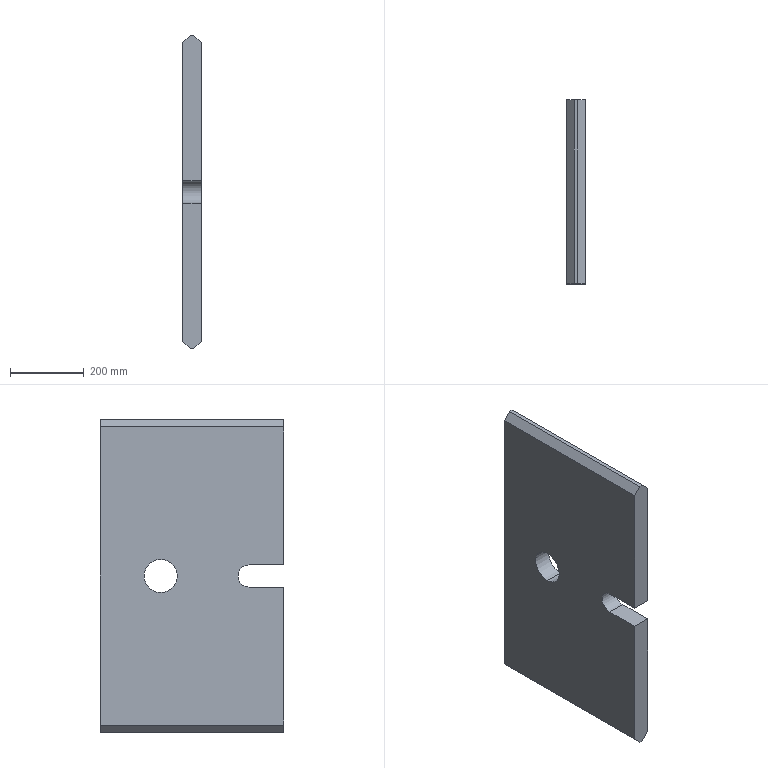Part | SolidWorks | features Chamfer 1, Extrusion 1 | 1 solid | 16 faces | box 50 x 500 x 850 mm | volume 20176228 mm3 | plane 13 | cylinder 3 | commonest cylinder face diameters 90 x2 60 x1
STEP:
#1=CARTESIAN_POINT('',(25.,85.,45.));
#2=VERTEX_POINT('',#1);
#3=CARTESIAN_POINT('',(25.,85.,-45.));
#4=VERTEX_POINT('',#3);
#5=CARTESIAN_POINT('',(25.,85.,0.));
#6=DIRECTION('',(1.,0.,0.));
#7=DIRECTION('',(0.,0.,-1.));
#8=AXIS2_PLACEMENT_3D('',#5,#6,#7);
#9=CIRCLE('',#8,45.);
#10=EDGE_CURVE('',#2,#4,#9,.T.);
#11=ORIENTED_EDGE('',*,*,#10,.T.);
#12=CARTESIAN_POINT('',(-25.,85.,-45.));
#13=VERTEX_POINT('',#12);
#14=CARTESIAN_POINT('',(25.,85.,-45.));
#15=DIRECTION('',(-1.,0.,0.));
#16=VECTOR('',#15,1000.);
#17=LINE('',#14,#16);
#18=EDGE_CURVE('',#4,#13,#17,.T.);
#19=ORIENTED_EDGE('',*,*,#18,.T.);
#20=CARTESIAN_POINT('',(-25.,85.,45.));
#21=VERTEX_POINT('',#20);
#22=CARTESIAN_POINT('',(-25.,85.,0.));
#23=DIRECTION('',(1.,0.,0.));
#24=DIRECTION('',(0.,0.,-1.));
#25=AXIS2_PLACEMENT_3D('',#22,#23,#24);
#26=CIRCLE('',#25,45.);
#27=EDGE_CURVE('',#21,#13,#26,.T.);
#28=ORIENTED_EDGE('',*,*,#27,.F.);
#29=CARTESIAN_POINT('',(25.,85.,45.));
#30=DIRECTION('',(-1.,0.,0.));
#31=VECTOR('',#30,1000.);
#32=LINE('',#29,#31);
#33=EDGE_CURVE('',#2,#21,#32,.T.);
#34=ORIENTED_EDGE('',*,*,#33,.F.);
#35=EDGE_LOOP('',(#11,#19,#28,#34));
#36=FACE_OUTER_BOUND('',#35,.T.);
#37=CARTESIAN_POINT('',(25.,85.,0.));
#38=DIRECTION('',(-1.,0.,0.));
#39=DIRECTION('',(0.,0.,1.));
#40=AXIS2_PLACEMENT_3D('',#37,#38,#39);
#41=CYLINDRICAL_SURFACE('',#40,45.);
#42=ADVANCED_FACE('',(#36),#41,.F.);
#43=CARTESIAN_POINT('',(25.,-250.,-30.));
#44=VERTEX_POINT('',#43);
#45=CARTESIAN_POINT('',(25.,-250.,-405.));
#46=VERTEX_POINT('',#45);
#47=CARTESIAN_POINT('',(25.,-250.,-425.));
#48=DIRECTION('',(0.,0.,-1.));
#49=VECTOR('',#48,1000.);
#50=LINE('',#47,#49);
#51=EDGE_CURVE('',#44,#46,#50,.T.);
#52=ORIENTED_EDGE('',*,*,#51,.T.);
#53=CARTESIAN_POINT('',(25.,250.,-405.));
#54=VERTEX_POINT('',#53);
#55=CARTESIAN_POINT('',(25.,250.,-405.));
#56=DIRECTION('',(0.,1.,0.));
#57=VECTOR('',#56,1000.);
#58=LINE('',#55,#57);
#59=EDGE_CURVE('',#46,#54,#58,.T.);
#60=ORIENTED_EDGE('',*,*,#59,.T.);
#61=CARTESIAN_POINT('',(25.,250.,405.));
#62=VERTEX_POINT('',#61);
#63=CARTESIAN_POINT('',(25.,250.,-425.));
#64=DIRECTION('',(0.,0.,1.));
#65=VECTOR('',#64,1000.);
#66=LINE('',#63,#65);
#67=EDGE_CURVE('',#54,#62,#66,.T.);
#68=ORIENTED_EDGE('',*,*,#67,.T.);
#69=CARTESIAN_POINT('',(25.,-250.,405.));
#70=VERTEX_POINT('',#69);
#71=CARTESIAN_POINT('',(25.,-250.,405.));
#72=DIRECTION('',(0.,-1.,0.));
#73=VECTOR('',#72,1000.);
#74=LINE('',#71,#73);
#75=EDGE_CURVE('',#62,#70,#74,.T.);
#76=ORIENTED_EDGE('',*,*,#75,.T.);
#77=CARTESIAN_POINT('',(25.,-250.,30.));
#78=VERTEX_POINT('',#77);
#79=CARTESIAN_POINT('',(25.,-250.,30.));
#80=DIRECTION('',(0.,0.,-1.));
#81=VECTOR('',#80,1000.);
#82=LINE('',#79,#81);
#83=EDGE_CURVE('',#70,#78,#82,.T.);
#84=ORIENTED_EDGE('',*,*,#83,.T.);
#85=CARTESIAN_POINT('',(25.,-155.,30.));
#86=VERTEX_POINT('',#85);
#87=CARTESIAN_POINT('',(25.,-155.,30.));
#88=DIRECTION('',(0.,1.,0.));
#89=VECTOR('',#88,1000.);
#90=LINE('',#87,#89);
#91=EDGE_CURVE('',#78,#86,#90,.T.);
#92=ORIENTED_EDGE('',*,*,#91,.T.);
#93=CARTESIAN_POINT('',(25.,-155.,-30.));
#94=VERTEX_POINT('',#93);
#95=CARTESIAN_POINT('',(25.,-155.,0.));
#96=DIRECTION('',(-1.,0.,0.));
#97=DIRECTION('',(0.,0.,-1.));
#98=AXIS2_PLACEMENT_3D('',#95,#96,#97);
#99=CIRCLE('',#98,30.);
#100=EDGE_CURVE('',#86,#94,#99,.T.);
#101=ORIENTED_EDGE('',*,*,#100,.T.);
#102=CARTESIAN_POINT('',(25.,-155.,-30.));
#103=DIRECTION('',(0.,-1.,0.));
#104=VECTOR('',#103,1000.);
#105=LINE('',#102,#104);
#106=EDGE_CURVE('',#94,#44,#105,.T.);
#107=ORIENTED_EDGE('',*,*,#106,.T.);
#108=EDGE_LOOP('',(#52,#60,#68,#76,#84,#92,#101,#107));
#109=FACE_OUTER_BOUND('',#108,.T.);
#110=ORIENTED_EDGE('',*,*,#10,.F.);
#111=CARTESIAN_POINT('',(25.,85.,0.));
#112=DIRECTION('',(1.,0.,0.));
#113=DIRECTION('',(0.,0.,-1.));
#114=AXIS2_PLACEMENT_3D('',#111,#112,#113);
#115=CIRCLE('',#114,45.);
#116=EDGE_CURVE('',#4,#2,#115,.T.);
#117=ORIENTED_EDGE('',*,*,#116,.F.);
#118=EDGE_LOOP('',(#110,#117));
#119=FACE_BOUND('',#118,.T.);
#120=CARTESIAN_POINT('',(25.,-155.,0.));
#121=DIRECTION('',(1.,0.,0.));
#122=DIRECTION('',(0.,0.,-1.));
#123=AXIS2_PLACEMENT_3D('',#120,#121,#122);
#124=PLANE('',#123);
#125=ADVANCED_FACE('',(#109,#119),#124,.T.);
#126=CARTESIAN_POINT('',(-25.,250.,-405.));
#127=VERTEX_POINT('',#126);
#128=CARTESIAN_POINT('',(-25.,250.,405.));
#129=VERTEX_POINT('',#128);
#130=CARTESIAN_POINT('',(-25.,250.,-425.));
#131=DIRECTION('',(0.,0.,1.));
#132=VECTOR('',#131,1000.);
#133=LINE('',#130,#132);
#134=EDGE_CURVE('',#127,#129,#133,.T.);
#135=ORIENTED_EDGE('',*,*,#134,.F.);
#136=CARTESIAN_POINT('',(-25.,-250.,-405.));
#137=VERTEX_POINT('',#136);
#138=CARTESIAN_POINT('',(-25.,-155.,-405.));
#139=DIRECTION('',(0.,-1.,0.));
#140=VECTOR('',#139,1000.);
#141=LINE('',#138,#140);
#142=EDGE_CURVE('',#127,#137,#141,.T.);
#143=ORIENTED_EDGE('',*,*,#142,.T.);
#144=CARTESIAN_POINT('',(-25.,-250.,-30.));
#145=VERTEX_POINT('',#144);
#146=CARTESIAN_POINT('',(-25.,-250.,-425.));
#147=DIRECTION('',(0.,0.,-1.));
#148=VECTOR('',#147,1000.);
#149=LINE('',#146,#148);
#150=EDGE_CURVE('',#145,#137,#149,.T.);
#151=ORIENTED_EDGE('',*,*,#150,.F.);
#152=CARTESIAN_POINT('',(-25.,-155.,-30.));
#153=VERTEX_POINT('',#152);
#154=CARTESIAN_POINT('',(-25.,-155.,-30.));
#155=DIRECTION('',(0.,-1.,0.));
#156=VECTOR('',#155,1000.);
#157=LINE('',#154,#156);
#158=EDGE_CURVE('',#153,#145,#157,.T.);
#159=ORIENTED_EDGE('',*,*,#158,.F.);
#160=CARTESIAN_POINT('',(-25.,-155.,30.));
#161=VERTEX_POINT('',#160);
#162=CARTESIAN_POINT('',(-25.,-155.,0.));
#163=DIRECTION('',(-1.,0.,0.));
#164=DIRECTION('',(0.,0.,-1.));
#165=AXIS2_PLACEMENT_3D('',#162,#163,#164);
#166=CIRCLE('',#165,30.);
#167=EDGE_CURVE('',#161,#153,#166,.T.);
#168=ORIENTED_EDGE('',*,*,#167,.F.);
#169=CARTESIAN_POINT('',(-25.,-250.,30.));
#170=VERTEX_POINT('',#169);
#171=CARTESIAN_POINT('',(-25.,-155.,30.));
#172=DIRECTION('',(0.,1.,0.));
#173=VECTOR('',#172,1000.);
#174=LINE('',#171,#173);
#175=EDGE_CURVE('',#170,#161,#174,.T.);
#176=ORIENTED_EDGE('',*,*,#175,.F.);
#177=CARTESIAN_POINT('',(-25.,-250.,405.));
#178=VERTEX_POINT('',#177);
#179=CARTESIAN_POINT('',(-25.,-250.,30.));
#180=DIRECTION('',(0.,0.,-1.));
#181=VECTOR('',#180,1000.);
#182=LINE('',#179,#181);
#183=EDGE_CURVE('',#178,#170,#182,.T.);
#184=ORIENTED_EDGE('',*,*,#183,.F.);
#185=CARTESIAN_POINT('',(-25.,-155.,405.));
#186=DIRECTION('',(0.,1.,0.));
#187=VECTOR('',#186,1000.);
#188=LINE('',#185,#187);
#189=EDGE_CURVE('',#178,#129,#188,.T.);
#190=ORIENTED_EDGE('',*,*,#189,.T.);
#191=EDGE_LOOP('',(#135,#143,#151,#159,#168,#176,#184,#190));
#192=FACE_OUTER_BOUND('',#191,.T.);
#193=ORIENTED_EDGE('',*,*,#27,.T.);
#194=CARTESIAN_POINT('',(-25.,85.,0.));
#195=DIRECTION('',(1.,0.,0.));
#196=DIRECTION('',(0.,0.,-1.));
#197=AXIS2_PLACEMENT_3D('',#194,#195,#196);
#198=CIRCLE('',#197,45.);
#199=EDGE_CURVE('',#13,#21,#198,.T.);
#200=ORIENTED_EDGE('',*,*,#199,.T.);
#201=EDGE_LOOP('',(#193,#200));
#202=FACE_BOUND('',#201,.T.);
#203=CARTESIAN_POINT('',(-25.,-155.,0.));
#204=DIRECTION('',(1.,0.,0.));
#205=DIRECTION('',(0.,0.,-1.));
#206=AXIS2_PLACEMENT_3D('',#203,#204,#205);
#207=PLANE('',#206);
#208=ADVANCED_FACE('',(#192,#202),#207,.F.);
#209=CARTESIAN_POINT('',(5.,250.,425.));
#210=VERTEX_POINT('',#209);
#211=CARTESIAN_POINT('',(-5.,250.,425.));
#212=VERTEX_POINT('',#211);
#213=CARTESIAN_POINT('',(25.,250.,425.));
#214=DIRECTION('',(-1.,0.,0.));
#215=VECTOR('',#214,1000.);
#216=LINE('',#213,#215);
#217=EDGE_CURVE('',#210,#212,#216,.T.);
#218=ORIENTED_EDGE('',*,*,#217,.T.);
#219=CARTESIAN_POINT('',(-5.,-250.,425.));
#220=VERTEX_POINT('',#219);
#221=CARTESIAN_POINT('',(-5.,-250.,425.));
#222=DIRECTION('',(0.,-1.,0.));
#223=VECTOR('',#222,1000.);
#224=LINE('',#221,#223);
#225=EDGE_CURVE('',#212,#220,#224,.T.);
#226=ORIENTED_EDGE('',*,*,#225,.T.);
#227=CARTESIAN_POINT('',(5.,-250.,425.));
#228=VERTEX_POINT('',#227);
#229=CARTESIAN_POINT('',(25.,-250.,425.));
#230=DIRECTION('',(-1.,0.,0.));
#231=VECTOR('',#230,1000.);
#232=LINE('',#229,#231);
#233=EDGE_CURVE('',#228,#220,#232,.T.);
#234=ORIENTED_EDGE('',*,*,#233,.F.);
#235=CARTESIAN_POINT('',(5.,250.,425.));
#236=DIRECTION('',(0.,1.,0.));
#237=VECTOR('',#236,1000.);
#238=LINE('',#235,#237);
#239=EDGE_CURVE('',#228,#210,#238,.T.);
#240=ORIENTED_EDGE('',*,*,#239,.T.);
#241=EDGE_LOOP('',(#218,#226,#234,#240));
#242=FACE_OUTER_BOUND('',#241,.T.);
#243=CARTESIAN_POINT('',(25.,-250.,425.));
#244=DIRECTION('',(0.,0.,-1.));
#245=DIRECTION('',(-1.,0.,0.));
#246=AXIS2_PLACEMENT_3D('',#243,#244,#245);
#247=PLANE('',#246);
#248=ADVANCED_FACE('',(#242),#247,.F.);
#249=ORIENTED_EDGE('',*,*,#233,.T.);
#250=CARTESIAN_POINT('',(-5.,-250.,425.));
#251=DIRECTION('',(-0.7071,0.,-0.7071));
#252=VECTOR('',#251,1000.);
#253=LINE('',#250,#252);
#254=EDGE_CURVE('',#220,#178,#253,.T.);
#255=ORIENTED_EDGE('',*,*,#254,.T.);
#256=ORIENTED_EDGE('',*,*,#183,.T.);
#257=CARTESIAN_POINT('',(25.,-250.,30.));
#258=DIRECTION('',(-1.,0.,0.));
#259=VECTOR('',#258,1000.);
#260=LINE('',#257,#259);
#261=EDGE_CURVE('',#78,#170,#260,.T.);
#262=ORIENTED_EDGE('',*,*,#261,.F.);
#263=ORIENTED_EDGE('',*,*,#83,.F.);
#264=CARTESIAN_POINT('',(25.,-250.,405.));
#265=DIRECTION('',(-0.7071,0.,0.7071));
#266=VECTOR('',#265,1000.);
#267=LINE('',#264,#266);
#268=EDGE_CURVE('',#70,#228,#267,.T.);
#269=ORIENTED_EDGE('',*,*,#268,.T.);
#270=EDGE_LOOP('',(#249,#255,#256,#262,#263,#269));
#271=FACE_OUTER_BOUND('',#270,.T.);
#272=CARTESIAN_POINT('',(25.,-250.,30.));
#273=DIRECTION('',(0.,1.,0.));
#274=DIRECTION('',(0.,0.,1.));
#275=AXIS2_PLACEMENT_3D('',#272,#273,#274);
#276=PLANE('',#275);
#277=ADVANCED_FACE('',(#271),#276,.F.);
#278=ORIENTED_EDGE('',*,*,#175,.T.);
#279=CARTESIAN_POINT('',(25.,-155.,30.));
#280=DIRECTION('',(-1.,0.,0.));
#281=VECTOR('',#280,1000.);
#282=LINE('',#279,#281);
#283=EDGE_CURVE('',#86,#161,#282,.T.);
#284=ORIENTED_EDGE('',*,*,#283,.F.);
#285=ORIENTED_EDGE('',*,*,#91,.F.);
#286=ORIENTED_EDGE('',*,*,#261,.T.);
#287=EDGE_LOOP('',(#278,#284,#285,#286));
#288=FACE_OUTER_BOUND('',#287,.T.);
#289=CARTESIAN_POINT('',(25.,-155.,30.));
#290=DIRECTION('',(0.,0.,1.));
#291=DIRECTION('',(1.,0.,0.));
#292=AXIS2_PLACEMENT_3D('',#289,#290,#291);
#293=PLANE('',#292);
#294=ADVANCED_FACE('',(#288),#293,.F.);
#295=ORIENTED_EDGE('',*,*,#167,.T.);
#296=CARTESIAN_POINT('',(25.,-155.,-30.));
#297=DIRECTION('',(-1.,0.,0.));
#298=VECTOR('',#297,1000.);
#299=LINE('',#296,#298);
#300=EDGE_CURVE('',#94,#153,#299,.T.);
#301=ORIENTED_EDGE('',*,*,#300,.F.);
#302=ORIENTED_EDGE('',*,*,#100,.F.);
#303=ORIENTED_EDGE('',*,*,#283,.T.);
#304=EDGE_LOOP('',(#295,#301,#302,#303));
#305=FACE_OUTER_BOUND('',#304,.T.);
#306=CARTESIAN_POINT('',(25.,-155.,0.));
#307=DIRECTION('',(-1.,0.,0.));
#308=DIRECTION('',(0.,0.,1.));
#309=AXIS2_PLACEMENT_3D('',#306,#307,#308);
#310=CYLINDRICAL_SURFACE('',#309,30.);
#311=ADVANCED_FACE('',(#305),#310,.F.);
#312=ORIENTED_EDGE('',*,*,#158,.T.);
#313=CARTESIAN_POINT('',(25.,-250.,-30.));
#314=DIRECTION('',(-1.,0.,0.));
#315=VECTOR('',#314,1000.);
#316=LINE('',#313,#315);
#317=EDGE_CURVE('',#44,#145,#316,.T.);
#318=ORIENTED_EDGE('',*,*,#317,.F.);
#319=ORIENTED_EDGE('',*,*,#106,.F.);
#320=ORIENTED_EDGE('',*,*,#300,.T.);
#321=EDGE_LOOP('',(#312,#318,#319,#320));
#322=FACE_OUTER_BOUND('',#321,.T.);
#323=CARTESIAN_POINT('',(25.,-155.,-30.));
#324=DIRECTION('',(0.,0.,-1.));
#325=DIRECTION('',(-1.,0.,0.));
#326=AXIS2_PLACEMENT_3D('',#323,#324,#325);
#327=PLANE('',#326);
#328=ADVANCED_FACE('',(#322),#327,.F.);
#329=ORIENTED_EDGE('',*,*,#150,.T.);
#330=CARTESIAN_POINT('',(-5.,-250.,-425.));
#331=VERTEX_POINT('',#330);
#332=CARTESIAN_POINT('',(-5.,-250.,-425.));
#333=DIRECTION('',(0.7071,0.,-0.7071));
#334=VECTOR('',#333,1000.);
#335=LINE('',#332,#334);
#336=EDGE_CURVE('',#137,#331,#335,.T.);
#337=ORIENTED_EDGE('',*,*,#336,.T.);
#338=CARTESIAN_POINT('',(5.,-250.,-425.));
#339=VERTEX_POINT('',#338);
#340=CARTESIAN_POINT('',(25.,-250.,-425.));
#341=DIRECTION('',(-1.,0.,0.));
#342=VECTOR('',#341,1000.);
#343=LINE('',#340,#342);
#344=EDGE_CURVE('',#339,#331,#343,.T.);
#345=ORIENTED_EDGE('',*,*,#344,.F.);
#346=CARTESIAN_POINT('',(25.,-250.,-405.));
#347=DIRECTION('',(0.7071,0.,0.7071));
#348=VECTOR('',#347,1000.);
#349=LINE('',#346,#348);
#350=EDGE_CURVE('',#339,#46,#349,.T.);
#351=ORIENTED_EDGE('',*,*,#350,.T.);
#352=ORIENTED_EDGE('',*,*,#51,.F.);
#353=ORIENTED_EDGE('',*,*,#317,.T.);
#354=EDGE_LOOP('',(#329,#337,#345,#351,#352,#353));
#355=FACE_OUTER_BOUND('',#354,.T.);
#356=CARTESIAN_POINT('',(25.,-250.,-425.));
#357=DIRECTION('',(0.,1.,0.));
#358=DIRECTION('',(0.,0.,1.));
#359=AXIS2_PLACEMENT_3D('',#356,#357,#358);
#360=PLANE('',#359);
#361=ADVANCED_FACE('',(#355),#360,.F.);
#362=ORIENTED_EDGE('',*,*,#344,.T.);
#363=CARTESIAN_POINT('',(-5.,250.,-425.));
#364=VERTEX_POINT('',#363);
#365=CARTESIAN_POINT('',(-5.,-250.,-425.));
#366=DIRECTION('',(0.,1.,0.));
#367=VECTOR('',#366,1000.);
#368=LINE('',#365,#367);
#369=EDGE_CURVE('',#331,#364,#368,.T.);
#370=ORIENTED_EDGE('',*,*,#369,.T.);
#371=CARTESIAN_POINT('',(5.,250.,-425.));
#372=VERTEX_POINT('',#371);
#373=CARTESIAN_POINT('',(25.,250.,-425.));
#374=DIRECTION('',(-1.,0.,0.));
#375=VECTOR('',#374,1000.);
#376=LINE('',#373,#375);
#377=EDGE_CURVE('',#372,#364,#376,.T.);
#378=ORIENTED_EDGE('',*,*,#377,.F.);
#379=CARTESIAN_POINT('',(5.,-250.,-425.));
#380=DIRECTION('',(0.,-1.,0.));
#381=VECTOR('',#380,1000.);
#382=LINE('',#379,#381);
#383=EDGE_CURVE('',#372,#339,#382,.T.);
#384=ORIENTED_EDGE('',*,*,#383,.T.);
#385=EDGE_LOOP('',(#362,#370,#378,#384));
#386=FACE_OUTER_BOUND('',#385,.T.);
#387=CARTESIAN_POINT('',(25.,-250.,-425.));
#388=DIRECTION('',(0.,0.,1.));
#389=DIRECTION('',(1.,0.,0.));
#390=AXIS2_PLACEMENT_3D('',#387,#388,#389);
#391=PLANE('',#390);
#392=ADVANCED_FACE('',(#386),#391,.F.);
#393=ORIENTED_EDGE('',*,*,#377,.T.);
#394=CARTESIAN_POINT('',(-5.,250.,-425.));
#395=DIRECTION('',(-0.7071,0.,0.7071));
#396=VECTOR('',#395,1000.);
#397=LINE('',#394,#396);
#398=EDGE_CURVE('',#364,#127,#397,.T.);
#399=ORIENTED_EDGE('',*,*,#398,.T.);
#400=ORIENTED_EDGE('',*,*,#134,.T.);
#401=CARTESIAN_POINT('',(-5.,250.,425.));
#402=DIRECTION('',(0.7071,0.,0.7071));
#403=VECTOR('',#402,1000.);
#404=LINE('',#401,#403);
#405=EDGE_CURVE('',#129,#212,#404,.T.);
#406=ORIENTED_EDGE('',*,*,#405,.T.);
#407=ORIENTED_EDGE('',*,*,#217,.F.);
#408=CARTESIAN_POINT('',(25.,250.,405.));
#409=DIRECTION('',(0.7071,0.,-0.7071));
#410=VECTOR('',#409,1000.);
#411=LINE('',#408,#410);
#412=EDGE_CURVE('',#210,#62,#411,.T.);
#413=ORIENTED_EDGE('',*,*,#412,.T.);
#414=ORIENTED_EDGE('',*,*,#67,.F.);
#415=CARTESIAN_POINT('',(25.,250.,-405.));
#416=DIRECTION('',(-0.7071,0.,-0.7071));
#417=VECTOR('',#416,1000.);
#418=LINE('',#415,#417);
#419=EDGE_CURVE('',#54,#372,#418,.T.);
#420=ORIENTED_EDGE('',*,*,#419,.T.);
#421=EDGE_LOOP('',(#393,#399,#400,#406,#407,#413,#414,#420));
#422=FACE_OUTER_BOUND('',#421,.T.);
#423=CARTESIAN_POINT('',(25.,250.,-425.));
#424=DIRECTION('',(0.,-1.,0.));
#425=DIRECTION('',(0.,0.,-1.));
#426=AXIS2_PLACEMENT_3D('',#423,#424,#425);
#427=PLANE('',#426);
#428=ADVANCED_FACE('',(#422),#427,.F.);
#429=ORIENTED_EDGE('',*,*,#18,.F.);
#430=ORIENTED_EDGE('',*,*,#116,.T.);
#431=ORIENTED_EDGE('',*,*,#33,.T.);
#432=ORIENTED_EDGE('',*,*,#199,.F.);
#433=EDGE_LOOP('',(#429,#430,#431,#432));
#434=FACE_OUTER_BOUND('',#433,.T.);
#435=CARTESIAN_POINT('',(25.,85.,0.));
#436=DIRECTION('',(-1.,0.,0.));
#437=DIRECTION('',(0.,0.,1.));
#438=AXIS2_PLACEMENT_3D('',#435,#436,#437);
#439=CYLINDRICAL_SURFACE('',#438,45.);
#440=ADVANCED_FACE('',(#434),#439,.F.);
#441=ORIENTED_EDGE('',*,*,#336,.F.);
#442=ORIENTED_EDGE('',*,*,#142,.F.);
#443=ORIENTED_EDGE('',*,*,#398,.F.);
#444=ORIENTED_EDGE('',*,*,#369,.F.);
#445=EDGE_LOOP('',(#441,#442,#443,#444));
#446=FACE_OUTER_BOUND('',#445,.T.);
#447=CARTESIAN_POINT('',(-5.,-250.,-425.));
#448=DIRECTION('',(0.7071,0.,0.7071));
#449=DIRECTION('',(0.,1.,0.));
#450=AXIS2_PLACEMENT_3D('',#447,#448,#449);
#451=PLANE('',#450);
#452=ADVANCED_FACE('',(#446),#451,.F.);
#453=ORIENTED_EDGE('',*,*,#350,.F.);
#454=ORIENTED_EDGE('',*,*,#383,.F.);
#455=ORIENTED_EDGE('',*,*,#419,.F.);
#456=ORIENTED_EDGE('',*,*,#59,.F.);
#457=EDGE_LOOP('',(#453,#454,#455,#456));
#458=FACE_OUTER_BOUND('',#457,.T.);
#459=CARTESIAN_POINT('',(25.,-155.,-405.));
#460=DIRECTION('',(0.7071,0.,-0.7071));
#461=DIRECTION('',(0.,-1.,0.));
#462=AXIS2_PLACEMENT_3D('',#459,#460,#461);
#463=PLANE('',#462);
#464=ADVANCED_FACE('',(#458),#463,.T.);
#465=ORIENTED_EDGE('',*,*,#405,.F.);
#466=ORIENTED_EDGE('',*,*,#189,.F.);
#467=ORIENTED_EDGE('',*,*,#254,.F.);
#468=ORIENTED_EDGE('',*,*,#225,.F.);
#469=EDGE_LOOP('',(#465,#466,#467,#468));
#470=FACE_OUTER_BOUND('',#469,.T.);
#471=CARTESIAN_POINT('',(-5.,-250.,425.));
#472=DIRECTION('',(0.7071,0.,-0.7071));
#473=DIRECTION('',(0.,-1.,0.));
#474=AXIS2_PLACEMENT_3D('',#471,#472,#473);
#475=PLANE('',#474);
#476=ADVANCED_FACE('',(#470),#475,.F.);
#477=ORIENTED_EDGE('',*,*,#412,.F.);
#478=ORIENTED_EDGE('',*,*,#239,.F.);
#479=ORIENTED_EDGE('',*,*,#268,.F.);
#480=ORIENTED_EDGE('',*,*,#75,.F.);
#481=EDGE_LOOP('',(#477,#478,#479,#480));
#482=FACE_OUTER_BOUND('',#481,.T.);
#483=CARTESIAN_POINT('',(25.,-155.,405.));
#484=DIRECTION('',(0.7071,0.,0.7071));
#485=DIRECTION('',(0.,1.,0.));
#486=AXIS2_PLACEMENT_3D('',#483,#484,#485);
#487=PLANE('',#486);
#488=ADVANCED_FACE('',(#482),#487,.T.);
#489=CLOSED_SHELL('',(#42,#125,#208,#248,#277,#294,#311,#328,#361,#392,#428,#440,#452,#464,#476,#488));
#490=MANIFOLD_SOLID_BREP('',#489);
#491=CARTESIAN_POINT('',(0.,0.,0.));
#492=DIRECTION('',(0.,0.,1.));
#493=DIRECTION('',(1.,0.,0.));
#494=AXIS2_PLACEMENT_3D('',#491,#492,#493);
#495=(LENGTH_UNIT()NAMED_UNIT(*)SI_UNIT(.MILLI.,.METRE.));
#496=UNCERTAINTY_MEASURE_WITH_UNIT(LENGTH_MEASURE(0.00001),#495,'','');
#497=(NAMED_UNIT(*)PLANE_ANGLE_UNIT()SI_UNIT($,.RADIAN.));
#498=(NAMED_UNIT(*)SI_UNIT($,.STERADIAN.)SOLID_ANGLE_UNIT());
#499=(GEOMETRIC_REPRESENTATION_CONTEXT(3)GLOBAL_UNCERTAINTY_ASSIGNED_CONTEXT((#496))GLOBAL_UNIT_ASSIGNED_CONTEXT((#495,#497,#498))REPRESENTATION_CONTEXT('',''));
#500=ADVANCED_BREP_SHAPE_REPRESENTATION('',(#490,#494),#499);